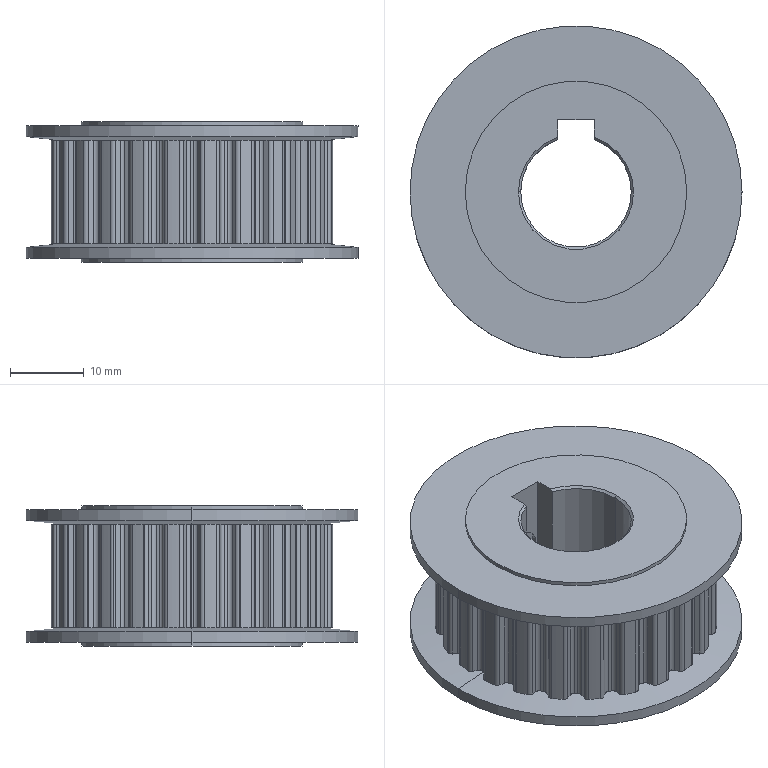Part | STEP file | EAF51-XL050-24-A-N-d15 | 1 solid | 369 faces | box 45 x 45 x 19 mm | volume 18328 mm3 | cylinder 182 | plane 173 | cone 14 | commonest cylinder face diameters 1.22 x116 35.5 x27 38.3 x24 4.134 x4 30 x4 45 x4